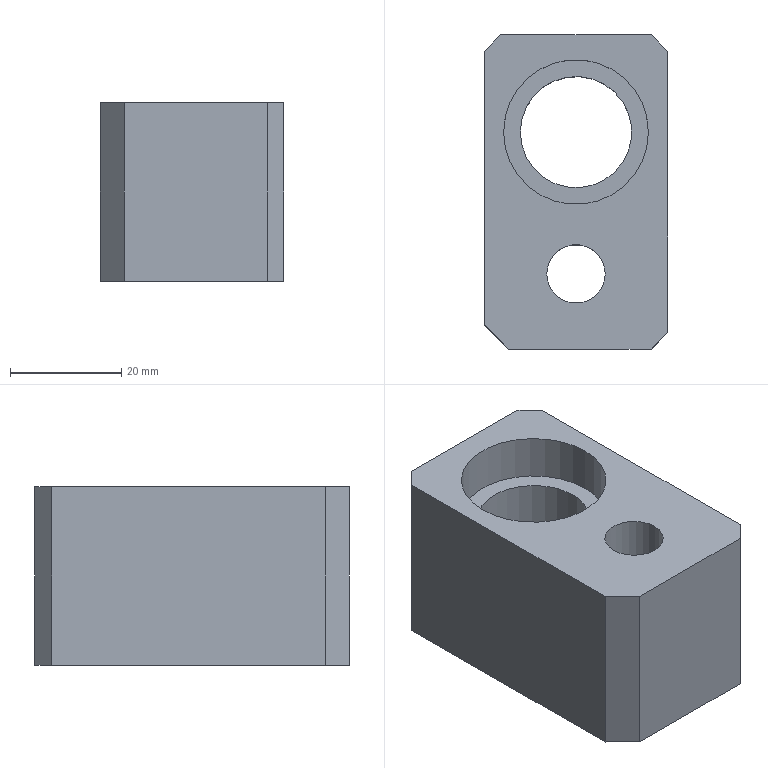Part | STEP file | lll_id3150_x_t | 1 solid | 16 faces | box 33 x 56.5 x 32 mm | volume 41942 mm3 | plane 12 | cylinder 4 | commonest cylinder face diameters 10.5 x1 17 x1 20 x1 26 x1
STEP:
#1=CARTESIAN_POINT('',(427.,-300.,60.5));
#2=VERTEX_POINT('',#1);
#3=CARTESIAN_POINT('',(437.,-300.,60.5));
#4=DIRECTION('',(0.,0.,1.));
#5=DIRECTION('',(-1.,0.,0.));
#6=AXIS2_PLACEMENT_3D('',#3,#4,#5);
#7=CIRCLE('',#6,10.);
#8=EDGE_CURVE('',#2,#2,#7,.T.);
#9=ORIENTED_EDGE('',*,*,#8,.T.);
#10=EDGE_LOOP('',(#9));
#11=FACE_BOUND('',#10,.T.);
#12=CARTESIAN_POINT('',(453.5,-336.,60.5));
#13=VERTEX_POINT('',#12);
#14=CARTESIAN_POINT('',(453.5,-285.5,60.5));
#15=VERTEX_POINT('',#14);
#16=CARTESIAN_POINT('',(453.5,-300.,60.5));
#17=DIRECTION('',(0.,1.,0.));
#18=VECTOR('',#17,1.);
#19=LINE('',#16,#18);
#20=EDGE_CURVE('',#13,#15,#19,.T.);
#21=ORIENTED_EDGE('',*,*,#20,.F.);
#22=CARTESIAN_POINT('',(450.5,-339.,60.5));
#23=VERTEX_POINT('',#22);
#24=CARTESIAN_POINT('',(411.067,-378.433,60.5));
#25=DIRECTION('',(-0.7071,-0.7071,0.));
#26=VECTOR('',#25,1.);
#27=LINE('',#24,#26);
#28=EDGE_CURVE('',#13,#23,#27,.T.);
#29=ORIENTED_EDGE('',*,*,#28,.T.);
#30=CARTESIAN_POINT('',(424.843,-339.,60.5));
#31=VERTEX_POINT('',#30);
#32=CARTESIAN_POINT('',(437.,-339.,60.5));
#33=DIRECTION('',(1.,0.,0.));
#34=VECTOR('',#33,1.);
#35=LINE('',#32,#34);
#36=EDGE_CURVE('',#31,#23,#35,.T.);
#37=ORIENTED_EDGE('',*,*,#36,.F.);
#38=CARTESIAN_POINT('',(420.5,-334.657,60.5));
#39=VERTEX_POINT('',#38);
#40=CARTESIAN_POINT('',(397.964,-312.121,60.5));
#41=DIRECTION('',(-0.7071,0.7071,0.));
#42=VECTOR('',#41,1.);
#43=LINE('',#40,#42);
#44=EDGE_CURVE('',#31,#39,#43,.T.);
#45=ORIENTED_EDGE('',*,*,#44,.T.);
#46=CARTESIAN_POINT('',(420.5,-285.5,60.5));
#47=VERTEX_POINT('',#46);
#48=CARTESIAN_POINT('',(420.5,-300.,60.5));
#49=DIRECTION('',(0.,-1.,0.));
#50=VECTOR('',#49,1.);
#51=LINE('',#48,#50);
#52=EDGE_CURVE('',#47,#39,#51,.T.);
#53=ORIENTED_EDGE('',*,*,#52,.F.);
#54=CARTESIAN_POINT('',(423.5,-282.5,60.5));
#55=VERTEX_POINT('',#54);
#56=CARTESIAN_POINT('',(371.817,-334.183,60.5));
#57=DIRECTION('',(0.7071,0.7071,0.));
#58=VECTOR('',#57,1.);
#59=LINE('',#56,#58);
#60=EDGE_CURVE('',#47,#55,#59,.T.);
#61=ORIENTED_EDGE('',*,*,#60,.T.);
#62=CARTESIAN_POINT('',(450.5,-282.5,60.5));
#63=VERTEX_POINT('',#62);
#64=CARTESIAN_POINT('',(437.,-282.5,60.5));
#65=DIRECTION('',(-1.,0.,0.));
#66=VECTOR('',#65,1.);
#67=LINE('',#64,#66);
#68=EDGE_CURVE('',#63,#55,#67,.T.);
#69=ORIENTED_EDGE('',*,*,#68,.F.);
#70=CARTESIAN_POINT('',(434.043,-266.043,60.5));
#71=DIRECTION('',(0.7071,-0.7071,0.));
#72=VECTOR('',#71,1.);
#73=LINE('',#70,#72);
#74=EDGE_CURVE('',#63,#15,#73,.T.);
#75=ORIENTED_EDGE('',*,*,#74,.T.);
#76=EDGE_LOOP('',(#21,#29,#37,#45,#53,#61,#69,#75));
#77=FACE_BOUND('',#76,.T.);
#78=CARTESIAN_POINT('',(445.5,-325.5,60.5));
#79=VERTEX_POINT('',#78);
#80=CARTESIAN_POINT('',(437.,-325.5,60.5));
#81=DIRECTION('',(0.,0.,1.));
#82=DIRECTION('',(1.,0.,0.));
#83=AXIS2_PLACEMENT_3D('',#80,#81,#82);
#84=CIRCLE('',#83,8.5);
#85=EDGE_CURVE('',#79,#79,#84,.T.);
#86=ORIENTED_EDGE('',*,*,#85,.T.);
#87=EDGE_LOOP('',(#86));
#88=FACE_BOUND('',#87,.T.);
#89=CARTESIAN_POINT('',(368.86,-331.225,60.5));
#90=DIRECTION('',(0.,0.,1.));
#91=DIRECTION('',(-1.,0.,0.));
#92=AXIS2_PLACEMENT_3D('',#89,#90,#91);
#93=PLANE('',#92);
#94=ADVANCED_FACE('',(#11,#77,#88),#93,.F.);
#95=CARTESIAN_POINT('',(450.,-300.,92.5));
#96=VERTEX_POINT('',#95);
#97=CARTESIAN_POINT('',(437.,-300.,92.5));
#98=DIRECTION('',(0.,0.,1.));
#99=DIRECTION('',(1.,0.,0.));
#100=AXIS2_PLACEMENT_3D('',#97,#98,#99);
#101=CIRCLE('',#100,13.);
#102=EDGE_CURVE('',#96,#96,#101,.T.);
#103=ORIENTED_EDGE('',*,*,#102,.F.);
#104=EDGE_LOOP('',(#103));
#105=FACE_BOUND('',#104,.T.);
#106=CARTESIAN_POINT('',(442.25,-325.5,92.5));
#107=VERTEX_POINT('',#106);
#108=CARTESIAN_POINT('',(437.,-325.5,92.5));
#109=DIRECTION('',(0.,0.,1.));
#110=DIRECTION('',(1.,0.,0.));
#111=AXIS2_PLACEMENT_3D('',#108,#109,#110);
#112=CIRCLE('',#111,5.25);
#113=EDGE_CURVE('',#107,#107,#112,.T.);
#114=ORIENTED_EDGE('',*,*,#113,.F.);
#115=EDGE_LOOP('',(#114));
#116=FACE_BOUND('',#115,.T.);
#117=CARTESIAN_POINT('',(450.5,-339.,92.5));
#118=VERTEX_POINT('',#117);
#119=CARTESIAN_POINT('',(424.843,-339.,92.5));
#120=VERTEX_POINT('',#119);
#121=CARTESIAN_POINT('',(437.,-339.,92.5));
#122=DIRECTION('',(-1.,0.,0.));
#123=VECTOR('',#122,1.);
#124=LINE('',#121,#123);
#125=EDGE_CURVE('',#118,#120,#124,.T.);
#126=ORIENTED_EDGE('',*,*,#125,.F.);
#127=CARTESIAN_POINT('',(453.5,-336.,92.5));
#128=VERTEX_POINT('',#127);
#129=CARTESIAN_POINT('',(411.067,-378.433,92.5));
#130=DIRECTION('',(0.7071,0.7071,0.));
#131=VECTOR('',#130,1.);
#132=LINE('',#129,#131);
#133=EDGE_CURVE('',#118,#128,#132,.T.);
#134=ORIENTED_EDGE('',*,*,#133,.T.);
#135=CARTESIAN_POINT('',(453.5,-285.5,92.5));
#136=VERTEX_POINT('',#135);
#137=CARTESIAN_POINT('',(453.5,-300.,92.5));
#138=DIRECTION('',(0.,-1.,0.));
#139=VECTOR('',#138,1.);
#140=LINE('',#137,#139);
#141=EDGE_CURVE('',#136,#128,#140,.T.);
#142=ORIENTED_EDGE('',*,*,#141,.F.);
#143=CARTESIAN_POINT('',(450.5,-282.5,92.5));
#144=VERTEX_POINT('',#143);
#145=CARTESIAN_POINT('',(434.043,-266.043,92.5));
#146=DIRECTION('',(-0.7071,0.7071,0.));
#147=VECTOR('',#146,1.);
#148=LINE('',#145,#147);
#149=EDGE_CURVE('',#136,#144,#148,.T.);
#150=ORIENTED_EDGE('',*,*,#149,.T.);
#151=CARTESIAN_POINT('',(423.5,-282.5,92.5));
#152=VERTEX_POINT('',#151);
#153=CARTESIAN_POINT('',(437.,-282.5,92.5));
#154=DIRECTION('',(1.,0.,0.));
#155=VECTOR('',#154,1.);
#156=LINE('',#153,#155);
#157=EDGE_CURVE('',#152,#144,#156,.T.);
#158=ORIENTED_EDGE('',*,*,#157,.F.);
#159=CARTESIAN_POINT('',(420.5,-285.5,92.5));
#160=VERTEX_POINT('',#159);
#161=CARTESIAN_POINT('',(371.817,-334.183,92.5));
#162=DIRECTION('',(-0.7071,-0.7071,0.));
#163=VECTOR('',#162,1.);
#164=LINE('',#161,#163);
#165=EDGE_CURVE('',#152,#160,#164,.T.);
#166=ORIENTED_EDGE('',*,*,#165,.T.);
#167=CARTESIAN_POINT('',(420.5,-334.657,92.5));
#168=VERTEX_POINT('',#167);
#169=CARTESIAN_POINT('',(420.5,-300.,92.5));
#170=DIRECTION('',(0.,1.,0.));
#171=VECTOR('',#170,1.);
#172=LINE('',#169,#171);
#173=EDGE_CURVE('',#168,#160,#172,.T.);
#174=ORIENTED_EDGE('',*,*,#173,.F.);
#175=CARTESIAN_POINT('',(397.964,-312.121,92.5));
#176=DIRECTION('',(0.7071,-0.7071,0.));
#177=VECTOR('',#176,1.);
#178=LINE('',#175,#177);
#179=EDGE_CURVE('',#168,#120,#178,.T.);
#180=ORIENTED_EDGE('',*,*,#179,.T.);
#181=EDGE_LOOP('',(#126,#134,#142,#150,#158,#166,#174,#180));
#182=FACE_BOUND('',#181,.T.);
#183=CARTESIAN_POINT('',(368.86,-331.225,92.5));
#184=DIRECTION('',(0.,0.,1.));
#185=DIRECTION('',(-1.,0.,0.));
#186=AXIS2_PLACEMENT_3D('',#183,#184,#185);
#187=PLANE('',#186);
#188=ADVANCED_FACE('',(#105,#116,#182),#187,.T.);
#189=ORIENTED_EDGE('',*,*,#157,.T.);
#190=CARTESIAN_POINT('',(450.5,-282.5,-8.5));
#191=DIRECTION('',(0.,0.,-1.));
#192=VECTOR('',#191,1.);
#193=LINE('',#190,#192);
#194=EDGE_CURVE('',#144,#63,#193,.T.);
#195=ORIENTED_EDGE('',*,*,#194,.T.);
#196=ORIENTED_EDGE('',*,*,#68,.T.);
#197=CARTESIAN_POINT('',(423.5,-282.5,-8.5));
#198=DIRECTION('',(0.,0.,1.));
#199=VECTOR('',#198,1.);
#200=LINE('',#197,#199);
#201=EDGE_CURVE('',#55,#152,#200,.T.);
#202=ORIENTED_EDGE('',*,*,#201,.T.);
#203=EDGE_LOOP('',(#189,#195,#196,#202));
#204=FACE_OUTER_BOUND('',#203,.T.);
#205=CARTESIAN_POINT('',(437.,-282.5,-8.5));
#206=DIRECTION('',(0.,1.,0.));
#207=DIRECTION('',(0.,0.,-1.));
#208=AXIS2_PLACEMENT_3D('',#205,#206,#207);
#209=PLANE('',#208);
#210=ADVANCED_FACE('',(#204),#209,.T.);
#211=ORIENTED_EDGE('',*,*,#141,.T.);
#212=CARTESIAN_POINT('',(453.5,-336.,-8.5));
#213=DIRECTION('',(0.,0.,-1.));
#214=VECTOR('',#213,1.);
#215=LINE('',#212,#214);
#216=EDGE_CURVE('',#128,#13,#215,.T.);
#217=ORIENTED_EDGE('',*,*,#216,.T.);
#218=ORIENTED_EDGE('',*,*,#20,.T.);
#219=CARTESIAN_POINT('',(453.5,-285.5,-8.5));
#220=DIRECTION('',(0.,0.,1.));
#221=VECTOR('',#220,1.);
#222=LINE('',#219,#221);
#223=EDGE_CURVE('',#15,#136,#222,.T.);
#224=ORIENTED_EDGE('',*,*,#223,.T.);
#225=EDGE_LOOP('',(#211,#217,#218,#224));
#226=FACE_OUTER_BOUND('',#225,.T.);
#227=CARTESIAN_POINT('',(453.5,-300.,-8.5));
#228=DIRECTION('',(1.,0.,0.));
#229=DIRECTION('',(0.,0.,1.));
#230=AXIS2_PLACEMENT_3D('',#227,#228,#229);
#231=PLANE('',#230);
#232=ADVANCED_FACE('',(#226),#231,.T.);
#233=ORIENTED_EDGE('',*,*,#36,.T.);
#234=CARTESIAN_POINT('',(450.5,-339.,-8.5));
#235=DIRECTION('',(0.,0.,1.));
#236=VECTOR('',#235,1.);
#237=LINE('',#234,#236);
#238=EDGE_CURVE('',#23,#118,#237,.T.);
#239=ORIENTED_EDGE('',*,*,#238,.T.);
#240=ORIENTED_EDGE('',*,*,#125,.T.);
#241=CARTESIAN_POINT('',(424.843,-339.,-8.5));
#242=DIRECTION('',(0.,0.,-1.));
#243=VECTOR('',#242,1.);
#244=LINE('',#241,#243);
#245=EDGE_CURVE('',#120,#31,#244,.T.);
#246=ORIENTED_EDGE('',*,*,#245,.T.);
#247=EDGE_LOOP('',(#233,#239,#240,#246));
#248=FACE_OUTER_BOUND('',#247,.T.);
#249=CARTESIAN_POINT('',(437.,-339.,-8.5));
#250=DIRECTION('',(0.,-1.,0.));
#251=DIRECTION('',(0.,0.,1.));
#252=AXIS2_PLACEMENT_3D('',#249,#250,#251);
#253=PLANE('',#252);
#254=ADVANCED_FACE('',(#248),#253,.T.);
#255=ORIENTED_EDGE('',*,*,#173,.T.);
#256=CARTESIAN_POINT('',(420.5,-285.5,-8.5));
#257=DIRECTION('',(0.,0.,-1.));
#258=VECTOR('',#257,1.);
#259=LINE('',#256,#258);
#260=EDGE_CURVE('',#160,#47,#259,.T.);
#261=ORIENTED_EDGE('',*,*,#260,.T.);
#262=ORIENTED_EDGE('',*,*,#52,.T.);
#263=CARTESIAN_POINT('',(420.5,-334.657,-8.5));
#264=DIRECTION('',(0.,0.,1.));
#265=VECTOR('',#264,1.);
#266=LINE('',#263,#265);
#267=EDGE_CURVE('',#39,#168,#266,.T.);
#268=ORIENTED_EDGE('',*,*,#267,.T.);
#269=EDGE_LOOP('',(#255,#261,#262,#268));
#270=FACE_OUTER_BOUND('',#269,.T.);
#271=CARTESIAN_POINT('',(420.5,-300.,-8.5));
#272=DIRECTION('',(-1.,0.,0.));
#273=DIRECTION('',(0.,0.,-1.));
#274=AXIS2_PLACEMENT_3D('',#271,#272,#273);
#275=PLANE('',#274);
#276=ADVANCED_FACE('',(#270),#275,.T.);
#277=ORIENTED_EDGE('',*,*,#113,.T.);
#278=EDGE_LOOP('',(#277));
#279=FACE_BOUND('',#278,.T.);
#280=CARTESIAN_POINT('',(442.25,-325.5,77.5));
#281=VERTEX_POINT('',#280);
#282=CARTESIAN_POINT('',(437.,-325.5,77.5));
#283=DIRECTION('',(0.,0.,-1.));
#284=DIRECTION('',(1.,0.,0.));
#285=AXIS2_PLACEMENT_3D('',#282,#283,#284);
#286=CIRCLE('',#285,5.25);
#287=EDGE_CURVE('',#281,#281,#286,.T.);
#288=ORIENTED_EDGE('',*,*,#287,.T.);
#289=EDGE_LOOP('',(#288));
#290=FACE_BOUND('',#289,.T.);
#291=CARTESIAN_POINT('',(437.,-325.5,160.5));
#292=DIRECTION('',(0.,0.,1.));
#293=DIRECTION('',(-1.,0.,0.));
#294=AXIS2_PLACEMENT_3D('',#291,#292,#293);
#295=CYLINDRICAL_SURFACE('',#294,5.25);
#296=ADVANCED_FACE('',(#279,#290),#295,.F.);
#297=ORIENTED_EDGE('',*,*,#287,.F.);
#298=EDGE_LOOP('',(#297));
#299=FACE_BOUND('',#298,.T.);
#300=CARTESIAN_POINT('',(445.5,-325.5,77.5));
#301=VERTEX_POINT('',#300);
#302=CARTESIAN_POINT('',(437.,-325.5,77.5));
#303=DIRECTION('',(0.,0.,-1.));
#304=DIRECTION('',(1.,0.,0.));
#305=AXIS2_PLACEMENT_3D('',#302,#303,#304);
#306=CIRCLE('',#305,8.5);
#307=EDGE_CURVE('',#301,#301,#306,.T.);
#308=ORIENTED_EDGE('',*,*,#307,.T.);
#309=EDGE_LOOP('',(#308));
#310=FACE_BOUND('',#309,.T.);
#311=CARTESIAN_POINT('',(437.,-325.5,77.5));
#312=DIRECTION('',(0.,0.,1.));
#313=DIRECTION('',(-1.,0.,0.));
#314=AXIS2_PLACEMENT_3D('',#311,#312,#313);
#315=PLANE('',#314);
#316=ADVANCED_FACE('',(#299,#310),#315,.F.);
#317=ORIENTED_EDGE('',*,*,#307,.F.);
#318=EDGE_LOOP('',(#317));
#319=FACE_BOUND('',#318,.T.);
#320=ORIENTED_EDGE('',*,*,#85,.F.);
#321=EDGE_LOOP('',(#320));
#322=FACE_BOUND('',#321,.T.);
#323=CARTESIAN_POINT('',(437.,-325.5,60.5));
#324=DIRECTION('',(0.,0.,1.));
#325=DIRECTION('',(-1.,0.,0.));
#326=AXIS2_PLACEMENT_3D('',#323,#324,#325);
#327=CYLINDRICAL_SURFACE('',#326,8.5);
#328=ADVANCED_FACE('',(#319,#322),#327,.F.);
#329=ORIENTED_EDGE('',*,*,#179,.F.);
#330=ORIENTED_EDGE('',*,*,#267,.F.);
#331=ORIENTED_EDGE('',*,*,#44,.F.);
#332=ORIENTED_EDGE('',*,*,#245,.F.);
#333=EDGE_LOOP('',(#329,#330,#331,#332));
#334=FACE_OUTER_BOUND('',#333,.T.);
#335=CARTESIAN_POINT('',(427.672,-341.828,-8.5));
#336=DIRECTION('',(0.7071,0.7071,0.));
#337=DIRECTION('',(0.,0.,-1.));
#338=AXIS2_PLACEMENT_3D('',#335,#336,#337);
#339=PLANE('',#338);
#340=ADVANCED_FACE('',(#334),#339,.F.);
#341=ORIENTED_EDGE('',*,*,#8,.F.);
#342=EDGE_LOOP('',(#341));
#343=FACE_BOUND('',#342,.T.);
#344=CARTESIAN_POINT('',(427.,-300.,84.3));
#345=VERTEX_POINT('',#344);
#346=CARTESIAN_POINT('',(437.,-300.,84.3));
#347=DIRECTION('',(0.,0.,-1.));
#348=DIRECTION('',(1.,0.,0.));
#349=AXIS2_PLACEMENT_3D('',#346,#347,#348);
#350=CIRCLE('',#349,10.);
#351=EDGE_CURVE('',#345,#345,#350,.T.);
#352=ORIENTED_EDGE('',*,*,#351,.F.);
#353=EDGE_LOOP('',(#352));
#354=FACE_BOUND('',#353,.T.);
#355=CARTESIAN_POINT('',(437.,-300.,124.8));
#356=DIRECTION('',(0.,0.,-1.));
#357=DIRECTION('',(1.,0.,0.));
#358=AXIS2_PLACEMENT_3D('',#355,#356,#357);
#359=CYLINDRICAL_SURFACE('',#358,10.);
#360=ADVANCED_FACE('',(#343,#354),#359,.F.);
#361=CARTESIAN_POINT('',(450.,-300.,84.3));
#362=VERTEX_POINT('',#361);
#363=CARTESIAN_POINT('',(437.,-300.,84.3));
#364=DIRECTION('',(0.,0.,1.));
#365=DIRECTION('',(1.,0.,0.));
#366=AXIS2_PLACEMENT_3D('',#363,#364,#365);
#367=CIRCLE('',#366,13.);
#368=EDGE_CURVE('',#362,#362,#367,.T.);
#369=ORIENTED_EDGE('',*,*,#368,.T.);
#370=EDGE_LOOP('',(#369));
#371=FACE_BOUND('',#370,.T.);
#372=ORIENTED_EDGE('',*,*,#351,.T.);
#373=EDGE_LOOP('',(#372));
#374=FACE_BOUND('',#373,.T.);
#375=CARTESIAN_POINT('',(437.,-300.,84.3));
#376=DIRECTION('',(0.,0.,1.));
#377=DIRECTION('',(-1.,0.,0.));
#378=AXIS2_PLACEMENT_3D('',#375,#376,#377);
#379=PLANE('',#378);
#380=ADVANCED_FACE('',(#371,#374),#379,.T.);
#381=ORIENTED_EDGE('',*,*,#368,.F.);
#382=EDGE_LOOP('',(#381));
#383=FACE_BOUND('',#382,.T.);
#384=ORIENTED_EDGE('',*,*,#102,.T.);
#385=EDGE_LOOP('',(#384));
#386=FACE_BOUND('',#385,.T.);
#387=CARTESIAN_POINT('',(437.,-300.,124.8));
#388=DIRECTION('',(0.,0.,-1.));
#389=DIRECTION('',(1.,0.,0.));
#390=AXIS2_PLACEMENT_3D('',#387,#388,#389);
#391=CYLINDRICAL_SURFACE('',#390,13.);
#392=ADVANCED_FACE('',(#383,#386),#391,.F.);
#393=ORIENTED_EDGE('',*,*,#74,.F.);
#394=ORIENTED_EDGE('',*,*,#194,.F.);
#395=ORIENTED_EDGE('',*,*,#149,.F.);
#396=ORIENTED_EDGE('',*,*,#223,.F.);
#397=EDGE_LOOP('',(#393,#394,#395,#396));
#398=FACE_OUTER_BOUND('',#397,.T.);
#399=CARTESIAN_POINT('',(453.5,-285.5,-8.5));
#400=DIRECTION('',(-0.7071,-0.7071,0.));
#401=DIRECTION('',(0.,0.,1.));
#402=AXIS2_PLACEMENT_3D('',#399,#400,#401);
#403=PLANE('',#402);
#404=ADVANCED_FACE('',(#398),#403,.F.);
#405=ORIENTED_EDGE('',*,*,#60,.F.);
#406=ORIENTED_EDGE('',*,*,#260,.F.);
#407=ORIENTED_EDGE('',*,*,#165,.F.);
#408=ORIENTED_EDGE('',*,*,#201,.F.);
#409=EDGE_LOOP('',(#405,#406,#407,#408));
#410=FACE_OUTER_BOUND('',#409,.T.);
#411=CARTESIAN_POINT('',(423.5,-282.5,-8.5));
#412=DIRECTION('',(0.7071,-0.7071,0.));
#413=DIRECTION('',(0.,0.,1.));
#414=AXIS2_PLACEMENT_3D('',#411,#412,#413);
#415=PLANE('',#414);
#416=ADVANCED_FACE('',(#410),#415,.F.);
#417=ORIENTED_EDGE('',*,*,#133,.F.);
#418=ORIENTED_EDGE('',*,*,#238,.F.);
#419=ORIENTED_EDGE('',*,*,#28,.F.);
#420=ORIENTED_EDGE('',*,*,#216,.F.);
#421=EDGE_LOOP('',(#417,#418,#419,#420));
#422=FACE_OUTER_BOUND('',#421,.T.);
#423=CARTESIAN_POINT('',(453.5,-336.,-8.5));
#424=DIRECTION('',(-0.7071,0.7071,0.));
#425=DIRECTION('',(0.,0.,-1.));
#426=AXIS2_PLACEMENT_3D('',#423,#424,#425);
#427=PLANE('',#426);
#428=ADVANCED_FACE('',(#422),#427,.F.);
#429=CLOSED_SHELL('',(#94,#188,#210,#232,#254,#276,#296,#316,#328,#340,#360,#380,#392,#404,#416,#428));
#430=MANIFOLD_SOLID_BREP('',#429);
#431=(LENGTH_UNIT()NAMED_UNIT(*)SI_UNIT(.MILLI.,.METRE.));
#432=UNCERTAINTY_MEASURE_WITH_UNIT(LENGTH_MEASURE(0.00002),#431,'','');
#433=(NAMED_UNIT(*)PLANE_ANGLE_UNIT()SI_UNIT($,.RADIAN.));
#434=PLANE_ANGLE_MEASURE_WITH_UNIT(PLANE_ANGLE_MEASURE(0.01745),#433);
#435=DIMENSIONAL_EXPONENTS(0.,0.,0.,0.,0.,0.,0.);
#436=(CONVERSION_BASED_UNIT('DEGREE',#434)NAMED_UNIT(#435)PLANE_ANGLE_UNIT());
#437=(NAMED_UNIT(*)SI_UNIT($,.STERADIAN.)SOLID_ANGLE_UNIT());
#438=(GEOMETRIC_REPRESENTATION_CONTEXT(3)GLOBAL_UNCERTAINTY_ASSIGNED_CONTEXT((#432))GLOBAL_UNIT_ASSIGNED_CONTEXT((#431,#436,#437))REPRESENTATION_CONTEXT('',''));
#439=ADVANCED_BREP_SHAPE_REPRESENTATION('',(#430),#438);